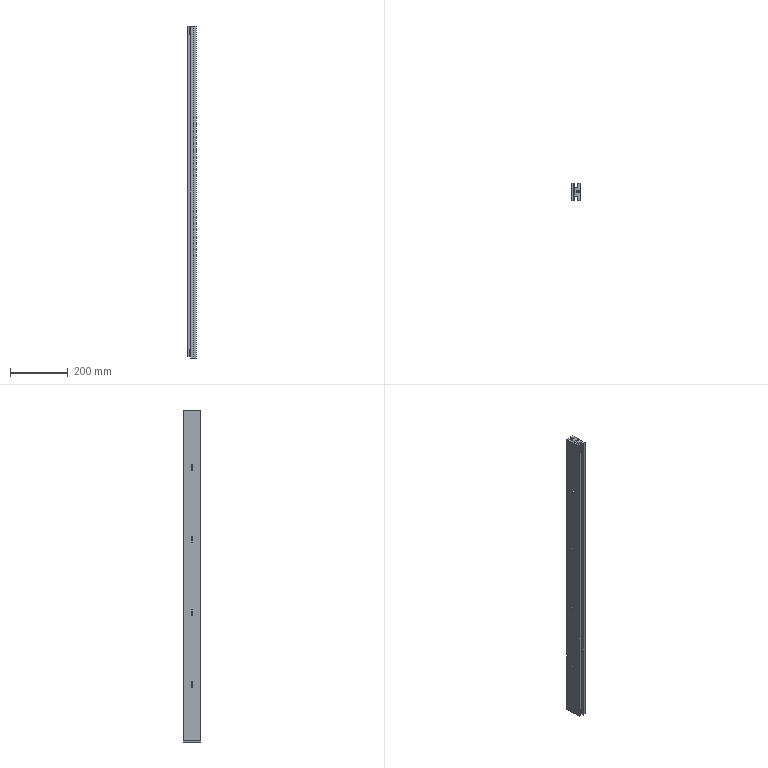Part | STEP file | 750038301 | 1 solid | 50 faces | box 30 x 60 x 1149 mm | volume 1566849 mm3 | plane 38 | cylinder 12 | commonest cylinder face diameters 6 x12
STEP:
#1=CARTESIAN_POINT('',(10.,30.,960.));
#2=VERTEX_POINT('',#1);
#3=CARTESIAN_POINT('',(10.,33.,957.));
#4=VERTEX_POINT('',#3);
#5=CARTESIAN_POINT('',(10.,30.,957.));
#6=DIRECTION('',(-1.,0.,0.));
#7=DIRECTION('',(0.,0.,1.));
#8=AXIS2_PLACEMENT_3D('',#5,#6,#7);
#9=CIRCLE('',#8,3.);
#10=EDGE_CURVE('',#2,#4,#9,.T.);
#11=ORIENTED_EDGE('',*,*,#10,.F.);
#12=CARTESIAN_POINT('',(0.,30.,960.));
#13=VERTEX_POINT('',#12);
#14=CARTESIAN_POINT('',(10.,30.,960.));
#15=DIRECTION('',(-1.,0.,0.));
#16=VECTOR('',#15,1000.);
#17=LINE('',#14,#16);
#18=EDGE_CURVE('',#2,#13,#17,.T.);
#19=ORIENTED_EDGE('',*,*,#18,.T.);
#20=CARTESIAN_POINT('',(0.,33.,957.));
#21=VERTEX_POINT('',#20);
#22=CARTESIAN_POINT('',(0.,30.,957.));
#23=DIRECTION('',(-1.,0.,0.));
#24=DIRECTION('',(0.,0.,1.));
#25=AXIS2_PLACEMENT_3D('',#22,#23,#24);
#26=CIRCLE('',#25,3.);
#27=EDGE_CURVE('',#13,#21,#26,.T.);
#28=ORIENTED_EDGE('',*,*,#27,.T.);
#29=CARTESIAN_POINT('',(10.,33.,957.));
#30=DIRECTION('',(-1.,0.,0.));
#31=VECTOR('',#30,1000.);
#32=LINE('',#29,#31);
#33=EDGE_CURVE('',#4,#21,#32,.T.);
#34=ORIENTED_EDGE('',*,*,#33,.F.);
#35=EDGE_LOOP('',(#11,#19,#28,#34));
#36=FACE_OUTER_BOUND('',#35,.T.);
#37=CARTESIAN_POINT('',(10.,30.,957.));
#38=DIRECTION('',(-1.,0.,0.));
#39=DIRECTION('',(0.,0.,1.));
#40=AXIS2_PLACEMENT_3D('',#37,#38,#39);
#41=CYLINDRICAL_SURFACE('',#40,3.);
#42=ADVANCED_FACE('',(#36),#41,.F.);
#43=CARTESIAN_POINT('',(10.,30.,710.));
#44=VERTEX_POINT('',#43);
#45=CARTESIAN_POINT('',(10.,33.,707.));
#46=VERTEX_POINT('',#45);
#47=CARTESIAN_POINT('',(10.,30.,707.));
#48=DIRECTION('',(-1.,0.,0.));
#49=DIRECTION('',(0.,0.,1.));
#50=AXIS2_PLACEMENT_3D('',#47,#48,#49);
#51=CIRCLE('',#50,3.);
#52=EDGE_CURVE('',#44,#46,#51,.T.);
#53=ORIENTED_EDGE('',*,*,#52,.F.);
#54=CARTESIAN_POINT('',(0.,30.,710.));
#55=VERTEX_POINT('',#54);
#56=CARTESIAN_POINT('',(10.,30.,710.));
#57=DIRECTION('',(-1.,0.,0.));
#58=VECTOR('',#57,1000.);
#59=LINE('',#56,#58);
#60=EDGE_CURVE('',#44,#55,#59,.T.);
#61=ORIENTED_EDGE('',*,*,#60,.T.);
#62=CARTESIAN_POINT('',(0.,33.,707.));
#63=VERTEX_POINT('',#62);
#64=CARTESIAN_POINT('',(0.,30.,707.));
#65=DIRECTION('',(-1.,0.,0.));
#66=DIRECTION('',(0.,0.,1.));
#67=AXIS2_PLACEMENT_3D('',#64,#65,#66);
#68=CIRCLE('',#67,3.);
#69=EDGE_CURVE('',#55,#63,#68,.T.);
#70=ORIENTED_EDGE('',*,*,#69,.T.);
#71=CARTESIAN_POINT('',(10.,33.,707.));
#72=DIRECTION('',(-1.,0.,0.));
#73=VECTOR('',#72,1000.);
#74=LINE('',#71,#73);
#75=EDGE_CURVE('',#46,#63,#74,.T.);
#76=ORIENTED_EDGE('',*,*,#75,.F.);
#77=EDGE_LOOP('',(#53,#61,#70,#76));
#78=FACE_OUTER_BOUND('',#77,.T.);
#79=CARTESIAN_POINT('',(10.,30.,707.));
#80=DIRECTION('',(-1.,0.,0.));
#81=DIRECTION('',(0.,0.,1.));
#82=AXIS2_PLACEMENT_3D('',#79,#80,#81);
#83=CYLINDRICAL_SURFACE('',#82,3.);
#84=ADVANCED_FACE('',(#78),#83,.F.);
#85=CARTESIAN_POINT('',(10.,30.,460.));
#86=VERTEX_POINT('',#85);
#87=CARTESIAN_POINT('',(10.,33.,457.));
#88=VERTEX_POINT('',#87);
#89=CARTESIAN_POINT('',(10.,30.,457.));
#90=DIRECTION('',(-1.,0.,0.));
#91=DIRECTION('',(0.,0.,1.));
#92=AXIS2_PLACEMENT_3D('',#89,#90,#91);
#93=CIRCLE('',#92,3.);
#94=EDGE_CURVE('',#86,#88,#93,.T.);
#95=ORIENTED_EDGE('',*,*,#94,.F.);
#96=CARTESIAN_POINT('',(0.,30.,460.));
#97=VERTEX_POINT('',#96);
#98=CARTESIAN_POINT('',(10.,30.,460.));
#99=DIRECTION('',(-1.,0.,0.));
#100=VECTOR('',#99,1000.);
#101=LINE('',#98,#100);
#102=EDGE_CURVE('',#86,#97,#101,.T.);
#103=ORIENTED_EDGE('',*,*,#102,.T.);
#104=CARTESIAN_POINT('',(0.,33.,457.));
#105=VERTEX_POINT('',#104);
#106=CARTESIAN_POINT('',(0.,30.,457.));
#107=DIRECTION('',(-1.,0.,0.));
#108=DIRECTION('',(0.,0.,1.));
#109=AXIS2_PLACEMENT_3D('',#106,#107,#108);
#110=CIRCLE('',#109,3.);
#111=EDGE_CURVE('',#97,#105,#110,.T.);
#112=ORIENTED_EDGE('',*,*,#111,.T.);
#113=CARTESIAN_POINT('',(10.,33.,457.));
#114=DIRECTION('',(-1.,0.,0.));
#115=VECTOR('',#114,1000.);
#116=LINE('',#113,#115);
#117=EDGE_CURVE('',#88,#105,#116,.T.);
#118=ORIENTED_EDGE('',*,*,#117,.F.);
#119=EDGE_LOOP('',(#95,#103,#112,#118));
#120=FACE_OUTER_BOUND('',#119,.T.);
#121=CARTESIAN_POINT('',(10.,30.,457.));
#122=DIRECTION('',(-1.,0.,0.));
#123=DIRECTION('',(0.,0.,1.));
#124=AXIS2_PLACEMENT_3D('',#121,#122,#123);
#125=CYLINDRICAL_SURFACE('',#124,3.);
#126=ADVANCED_FACE('',(#120),#125,.F.);
#127=CARTESIAN_POINT('',(10.,30.,210.));
#128=VERTEX_POINT('',#127);
#129=CARTESIAN_POINT('',(10.,33.,207.));
#130=VERTEX_POINT('',#129);
#131=CARTESIAN_POINT('',(10.,30.,207.));
#132=DIRECTION('',(-1.,0.,0.));
#133=DIRECTION('',(0.,0.,1.));
#134=AXIS2_PLACEMENT_3D('',#131,#132,#133);
#135=CIRCLE('',#134,3.);
#136=EDGE_CURVE('',#128,#130,#135,.T.);
#137=ORIENTED_EDGE('',*,*,#136,.F.);
#138=CARTESIAN_POINT('',(0.,30.,210.));
#139=VERTEX_POINT('',#138);
#140=CARTESIAN_POINT('',(10.,30.,210.));
#141=DIRECTION('',(-1.,0.,0.));
#142=VECTOR('',#141,1000.);
#143=LINE('',#140,#142);
#144=EDGE_CURVE('',#128,#139,#143,.T.);
#145=ORIENTED_EDGE('',*,*,#144,.T.);
#146=CARTESIAN_POINT('',(0.,33.,207.));
#147=VERTEX_POINT('',#146);
#148=CARTESIAN_POINT('',(0.,30.,207.));
#149=DIRECTION('',(-1.,0.,0.));
#150=DIRECTION('',(0.,0.,1.));
#151=AXIS2_PLACEMENT_3D('',#148,#149,#150);
#152=CIRCLE('',#151,3.);
#153=EDGE_CURVE('',#139,#147,#152,.T.);
#154=ORIENTED_EDGE('',*,*,#153,.T.);
#155=CARTESIAN_POINT('',(10.,33.,207.));
#156=DIRECTION('',(-1.,0.,0.));
#157=VECTOR('',#156,1000.);
#158=LINE('',#155,#157);
#159=EDGE_CURVE('',#130,#147,#158,.T.);
#160=ORIENTED_EDGE('',*,*,#159,.F.);
#161=EDGE_LOOP('',(#137,#145,#154,#160));
#162=FACE_OUTER_BOUND('',#161,.T.);
#163=CARTESIAN_POINT('',(10.,30.,207.));
#164=DIRECTION('',(-1.,0.,0.));
#165=DIRECTION('',(0.,0.,1.));
#166=AXIS2_PLACEMENT_3D('',#163,#164,#165);
#167=CYLINDRICAL_SURFACE('',#166,3.);
#168=ADVANCED_FACE('',(#162),#167,.F.);
#169=CARTESIAN_POINT('',(0.,0.,1149.));
#170=VERTEX_POINT('',#169);
#171=CARTESIAN_POINT('',(0.,0.,5.));
#172=VERTEX_POINT('',#171);
#173=CARTESIAN_POINT('',(0.,0.,1149.));
#174=DIRECTION('',(0.,0.,-1.));
#175=VECTOR('',#174,1000.);
#176=LINE('',#173,#175);
#177=EDGE_CURVE('',#170,#172,#176,.T.);
#178=ORIENTED_EDGE('',*,*,#177,.F.);
#179=CARTESIAN_POINT('',(0.,60.,1149.));
#180=VERTEX_POINT('',#179);
#181=CARTESIAN_POINT('',(0.,60.,1149.));
#182=DIRECTION('',(0.,-1.,0.));
#183=VECTOR('',#182,1000.);
#184=LINE('',#181,#183);
#185=EDGE_CURVE('',#180,#170,#184,.T.);
#186=ORIENTED_EDGE('',*,*,#185,.F.);
#187=CARTESIAN_POINT('',(0.,60.,5.));
#188=VERTEX_POINT('',#187);
#189=CARTESIAN_POINT('',(0.,60.,1149.));
#190=DIRECTION('',(0.,0.,1.));
#191=VECTOR('',#190,1000.);
#192=LINE('',#189,#191);
#193=EDGE_CURVE('',#188,#180,#192,.T.);
#194=ORIENTED_EDGE('',*,*,#193,.F.);
#195=CARTESIAN_POINT('',(0.,60.,5.));
#196=DIRECTION('',(0.,1.,0.));
#197=VECTOR('',#196,1000.);
#198=LINE('',#195,#197);
#199=EDGE_CURVE('',#172,#188,#198,.T.);
#200=ORIENTED_EDGE('',*,*,#199,.F.);
#201=EDGE_LOOP('',(#178,#186,#194,#200));
#202=FACE_OUTER_BOUND('',#201,.T.);
#203=CARTESIAN_POINT('',(0.,27.,942.));
#204=VERTEX_POINT('',#203);
#205=CARTESIAN_POINT('',(0.,27.,957.));
#206=VERTEX_POINT('',#205);
#207=CARTESIAN_POINT('',(0.,27.,1149.));
#208=DIRECTION('',(0.,0.,1.));
#209=VECTOR('',#208,1000.);
#210=LINE('',#207,#209);
#211=EDGE_CURVE('',#204,#206,#210,.T.);
#212=ORIENTED_EDGE('',*,*,#211,.F.);
#213=CARTESIAN_POINT('',(0.,33.,942.));
#214=VERTEX_POINT('',#213);
#215=CARTESIAN_POINT('',(0.,30.,942.));
#216=DIRECTION('',(-1.,0.,0.));
#217=DIRECTION('',(0.,0.,1.));
#218=AXIS2_PLACEMENT_3D('',#215,#216,#217);
#219=CIRCLE('',#218,3.);
#220=EDGE_CURVE('',#214,#204,#219,.T.);
#221=ORIENTED_EDGE('',*,*,#220,.F.);
#222=CARTESIAN_POINT('',(0.,33.,1149.));
#223=DIRECTION('',(0.,0.,-1.));
#224=VECTOR('',#223,1000.);
#225=LINE('',#222,#224);
#226=EDGE_CURVE('',#21,#214,#225,.T.);
#227=ORIENTED_EDGE('',*,*,#226,.F.);
#228=ORIENTED_EDGE('',*,*,#27,.F.);
#229=CARTESIAN_POINT('',(0.,30.,957.));
#230=DIRECTION('',(-1.,0.,0.));
#231=DIRECTION('',(0.,0.,1.));
#232=AXIS2_PLACEMENT_3D('',#229,#230,#231);
#233=CIRCLE('',#232,3.);
#234=EDGE_CURVE('',#206,#13,#233,.T.);
#235=ORIENTED_EDGE('',*,*,#234,.F.);
#236=EDGE_LOOP('',(#212,#221,#227,#228,#235));
#237=FACE_BOUND('',#236,.T.);
#238=CARTESIAN_POINT('',(0.,27.,692.));
#239=VERTEX_POINT('',#238);
#240=CARTESIAN_POINT('',(0.,27.,707.));
#241=VERTEX_POINT('',#240);
#242=CARTESIAN_POINT('',(0.,27.,1149.));
#243=DIRECTION('',(0.,0.,1.));
#244=VECTOR('',#243,1000.);
#245=LINE('',#242,#244);
#246=EDGE_CURVE('',#239,#241,#245,.T.);
#247=ORIENTED_EDGE('',*,*,#246,.F.);
#248=CARTESIAN_POINT('',(0.,33.,692.));
#249=VERTEX_POINT('',#248);
#250=CARTESIAN_POINT('',(0.,30.,692.));
#251=DIRECTION('',(-1.,0.,0.));
#252=DIRECTION('',(0.,0.,1.));
#253=AXIS2_PLACEMENT_3D('',#250,#251,#252);
#254=CIRCLE('',#253,3.);
#255=EDGE_CURVE('',#249,#239,#254,.T.);
#256=ORIENTED_EDGE('',*,*,#255,.F.);
#257=CARTESIAN_POINT('',(0.,33.,1149.));
#258=DIRECTION('',(0.,0.,-1.));
#259=VECTOR('',#258,1000.);
#260=LINE('',#257,#259);
#261=EDGE_CURVE('',#63,#249,#260,.T.);
#262=ORIENTED_EDGE('',*,*,#261,.F.);
#263=ORIENTED_EDGE('',*,*,#69,.F.);
#264=CARTESIAN_POINT('',(0.,30.,707.));
#265=DIRECTION('',(-1.,0.,0.));
#266=DIRECTION('',(0.,0.,1.));
#267=AXIS2_PLACEMENT_3D('',#264,#265,#266);
#268=CIRCLE('',#267,3.);
#269=EDGE_CURVE('',#241,#55,#268,.T.);
#270=ORIENTED_EDGE('',*,*,#269,.F.);
#271=EDGE_LOOP('',(#247,#256,#262,#263,#270));
#272=FACE_BOUND('',#271,.T.);
#273=CARTESIAN_POINT('',(0.,27.,442.));
#274=VERTEX_POINT('',#273);
#275=CARTESIAN_POINT('',(0.,27.,457.));
#276=VERTEX_POINT('',#275);
#277=CARTESIAN_POINT('',(0.,27.,1149.));
#278=DIRECTION('',(0.,0.,1.));
#279=VECTOR('',#278,1000.);
#280=LINE('',#277,#279);
#281=EDGE_CURVE('',#274,#276,#280,.T.);
#282=ORIENTED_EDGE('',*,*,#281,.F.);
#283=CARTESIAN_POINT('',(0.,33.,442.));
#284=VERTEX_POINT('',#283);
#285=CARTESIAN_POINT('',(0.,30.,442.));
#286=DIRECTION('',(-1.,0.,0.));
#287=DIRECTION('',(0.,0.,1.));
#288=AXIS2_PLACEMENT_3D('',#285,#286,#287);
#289=CIRCLE('',#288,3.);
#290=EDGE_CURVE('',#284,#274,#289,.T.);
#291=ORIENTED_EDGE('',*,*,#290,.F.);
#292=CARTESIAN_POINT('',(0.,33.,1149.));
#293=DIRECTION('',(0.,0.,-1.));
#294=VECTOR('',#293,1000.);
#295=LINE('',#292,#294);
#296=EDGE_CURVE('',#105,#284,#295,.T.);
#297=ORIENTED_EDGE('',*,*,#296,.F.);
#298=ORIENTED_EDGE('',*,*,#111,.F.);
#299=CARTESIAN_POINT('',(0.,30.,457.));
#300=DIRECTION('',(-1.,0.,0.));
#301=DIRECTION('',(0.,0.,1.));
#302=AXIS2_PLACEMENT_3D('',#299,#300,#301);
#303=CIRCLE('',#302,3.);
#304=EDGE_CURVE('',#276,#97,#303,.T.);
#305=ORIENTED_EDGE('',*,*,#304,.F.);
#306=EDGE_LOOP('',(#282,#291,#297,#298,#305));
#307=FACE_BOUND('',#306,.T.);
#308=CARTESIAN_POINT('',(0.,27.,192.));
#309=VERTEX_POINT('',#308);
#310=CARTESIAN_POINT('',(0.,27.,207.));
#311=VERTEX_POINT('',#310);
#312=CARTESIAN_POINT('',(0.,27.,1149.));
#313=DIRECTION('',(0.,0.,1.));
#314=VECTOR('',#313,1000.);
#315=LINE('',#312,#314);
#316=EDGE_CURVE('',#309,#311,#315,.T.);
#317=ORIENTED_EDGE('',*,*,#316,.F.);
#318=CARTESIAN_POINT('',(0.,33.,192.));
#319=VERTEX_POINT('',#318);
#320=CARTESIAN_POINT('',(0.,30.,192.));
#321=DIRECTION('',(-1.,0.,0.));
#322=DIRECTION('',(0.,0.,1.));
#323=AXIS2_PLACEMENT_3D('',#320,#321,#322);
#324=CIRCLE('',#323,3.);
#325=EDGE_CURVE('',#319,#309,#324,.T.);
#326=ORIENTED_EDGE('',*,*,#325,.F.);
#327=CARTESIAN_POINT('',(0.,33.,1149.));
#328=DIRECTION('',(0.,0.,-1.));
#329=VECTOR('',#328,1000.);
#330=LINE('',#327,#329);
#331=EDGE_CURVE('',#147,#319,#330,.T.);
#332=ORIENTED_EDGE('',*,*,#331,.F.);
#333=ORIENTED_EDGE('',*,*,#153,.F.);
#334=CARTESIAN_POINT('',(0.,30.,207.));
#335=DIRECTION('',(-1.,0.,0.));
#336=DIRECTION('',(0.,0.,1.));
#337=AXIS2_PLACEMENT_3D('',#334,#335,#336);
#338=CIRCLE('',#337,3.);
#339=EDGE_CURVE('',#311,#139,#338,.T.);
#340=ORIENTED_EDGE('',*,*,#339,.F.);
#341=EDGE_LOOP('',(#317,#326,#332,#333,#340));
#342=FACE_BOUND('',#341,.T.);
#343=CARTESIAN_POINT('',(0.,60.,1149.));
#344=DIRECTION('',(1.,0.,0.));
#345=DIRECTION('',(0.,0.,-1.));
#346=AXIS2_PLACEMENT_3D('',#343,#344,#345);
#347=PLANE('',#346);
#348=ADVANCED_FACE('',(#202,#237,#272,#307,#342),#347,.F.);
#349=CARTESIAN_POINT('',(6.5,0.,5.));
#350=VERTEX_POINT('',#349);
#351=CARTESIAN_POINT('',(10.,0.,5.));
#352=DIRECTION('',(1.,0.,0.));
#353=VECTOR('',#352,1000.);
#354=LINE('',#351,#353);
#355=EDGE_CURVE('',#172,#350,#354,.T.);
#356=ORIENTED_EDGE('',*,*,#355,.F.);
#357=ORIENTED_EDGE('',*,*,#199,.T.);
#358=CARTESIAN_POINT('',(6.5,60.,5.));
#359=VERTEX_POINT('',#358);
#360=CARTESIAN_POINT('',(10.,60.,5.));
#361=DIRECTION('',(-1.,0.,0.));
#362=VECTOR('',#361,1000.);
#363=LINE('',#360,#362);
#364=EDGE_CURVE('',#359,#188,#363,.T.);
#365=ORIENTED_EDGE('',*,*,#364,.F.);
#366=CARTESIAN_POINT('',(6.5,0.,5.));
#367=DIRECTION('',(0.,1.,0.));
#368=VECTOR('',#367,1000.);
#369=LINE('',#366,#368);
#370=EDGE_CURVE('',#350,#359,#369,.T.);
#371=ORIENTED_EDGE('',*,*,#370,.F.);
#372=EDGE_LOOP('',(#356,#357,#365,#371));
#373=FACE_OUTER_BOUND('',#372,.T.);
#374=CARTESIAN_POINT('',(10.,0.,5.));
#375=DIRECTION('',(0.,0.,1.));
#376=DIRECTION('',(0.,-1.,0.));
#377=AXIS2_PLACEMENT_3D('',#374,#375,#376);
#378=PLANE('',#377);
#379=ADVANCED_FACE('',(#373),#378,.F.);
#380=CARTESIAN_POINT('',(6.5,0.,1118.));
#381=VERTEX_POINT('',#380);
#382=CARTESIAN_POINT('',(9.5,0.,1118.));
#383=VERTEX_POINT('',#382);
#384=CARTESIAN_POINT('',(0.,0.,1118.));
#385=DIRECTION('',(1.,0.,0.));
#386=VECTOR('',#385,1000.);
#387=LINE('',#384,#386);
#388=EDGE_CURVE('',#381,#383,#387,.T.);
#389=ORIENTED_EDGE('',*,*,#388,.F.);
#390=CARTESIAN_POINT('',(6.5,0.,1149.));
#391=VERTEX_POINT('',#390);
#392=CARTESIAN_POINT('',(6.5,0.,1149.));
#393=DIRECTION('',(0.,0.,-1.));
#394=VECTOR('',#393,1000.);
#395=LINE('',#392,#394);
#396=EDGE_CURVE('',#391,#381,#395,.T.);
#397=ORIENTED_EDGE('',*,*,#396,.F.);
#398=CARTESIAN_POINT('',(0.,0.,1149.));
#399=DIRECTION('',(1.,0.,0.));
#400=VECTOR('',#399,1000.);
#401=LINE('',#398,#400);
#402=EDGE_CURVE('',#170,#391,#401,.T.);
#403=ORIENTED_EDGE('',*,*,#402,.F.);
#404=ORIENTED_EDGE('',*,*,#177,.T.);
#405=ORIENTED_EDGE('',*,*,#355,.T.);
#406=CARTESIAN_POINT('',(6.5,0.,31.));
#407=VERTEX_POINT('',#406);
#408=CARTESIAN_POINT('',(6.5,0.,1149.));
#409=DIRECTION('',(0.,0.,-1.));
#410=VECTOR('',#409,1000.);
#411=LINE('',#408,#410);
#412=EDGE_CURVE('',#407,#350,#411,.T.);
#413=ORIENTED_EDGE('',*,*,#412,.F.);
#414=CARTESIAN_POINT('',(9.5,0.,31.));
#415=VERTEX_POINT('',#414);
#416=CARTESIAN_POINT('',(0.,0.,31.));
#417=DIRECTION('',(-1.,0.,0.));
#418=VECTOR('',#417,1000.);
#419=LINE('',#416,#418);
#420=EDGE_CURVE('',#415,#407,#419,.T.);
#421=ORIENTED_EDGE('',*,*,#420,.F.);
#422=CARTESIAN_POINT('',(9.5,0.,1149.));
#423=DIRECTION('',(0.,0.,-1.));
#424=VECTOR('',#423,1000.);
#425=LINE('',#422,#424);
#426=EDGE_CURVE('',#383,#415,#425,.T.);
#427=ORIENTED_EDGE('',*,*,#426,.F.);
#428=EDGE_LOOP('',(#389,#397,#403,#404,#405,#413,#421,#427));
#429=FACE_OUTER_BOUND('',#428,.T.);
#430=CARTESIAN_POINT('',(0.,0.,1149.));
#431=DIRECTION('',(0.,1.,0.));
#432=DIRECTION('',(0.,0.,1.));
#433=AXIS2_PLACEMENT_3D('',#430,#431,#432);
#434=PLANE('',#433);
#435=ADVANCED_FACE('',(#429),#434,.F.);
#436=CARTESIAN_POINT('',(6.5,60.,1149.));
#437=VERTEX_POINT('',#436);
#438=CARTESIAN_POINT('',(0.,60.,1149.));
#439=DIRECTION('',(-1.,0.,0.));
#440=VECTOR('',#439,1000.);
#441=LINE('',#438,#440);
#442=EDGE_CURVE('',#437,#180,#441,.T.);
#443=ORIENTED_EDGE('',*,*,#442,.T.);
#444=ORIENTED_EDGE('',*,*,#185,.T.);
#445=ORIENTED_EDGE('',*,*,#402,.T.);
#446=CARTESIAN_POINT('',(6.5,0.,1149.));
#447=DIRECTION('',(0.,1.,0.));
#448=VECTOR('',#447,1000.);
#449=LINE('',#446,#448);
#450=EDGE_CURVE('',#391,#437,#449,.T.);
#451=ORIENTED_EDGE('',*,*,#450,.T.);
#452=EDGE_LOOP('',(#443,#444,#445,#451));
#453=FACE_OUTER_BOUND('',#452,.T.);
#454=CARTESIAN_POINT('',(0.,0.,1149.));
#455=DIRECTION('',(0.,0.,1.));
#456=DIRECTION('',(1.,0.,0.));
#457=AXIS2_PLACEMENT_3D('',#454,#455,#456);
#458=PLANE('',#457);
#459=ADVANCED_FACE('',(#453),#458,.T.);
#460=CARTESIAN_POINT('',(9.5,60.,1118.));
#461=VERTEX_POINT('',#460);
#462=CARTESIAN_POINT('',(6.5,60.,1118.));
#463=VERTEX_POINT('',#462);
#464=CARTESIAN_POINT('',(9.5,60.,1118.));
#465=DIRECTION('',(-1.,0.,0.));
#466=VECTOR('',#465,1000.);
#467=LINE('',#464,#466);
#468=EDGE_CURVE('',#461,#463,#467,.T.);
#469=ORIENTED_EDGE('',*,*,#468,.F.);
#470=CARTESIAN_POINT('',(9.5,60.,31.));
#471=VERTEX_POINT('',#470);
#472=CARTESIAN_POINT('',(9.5,60.,1149.));
#473=DIRECTION('',(0.,0.,1.));
#474=VECTOR('',#473,1000.);
#475=LINE('',#472,#474);
#476=EDGE_CURVE('',#471,#461,#475,.T.);
#477=ORIENTED_EDGE('',*,*,#476,.F.);
#478=CARTESIAN_POINT('',(6.5,60.,31.));
#479=VERTEX_POINT('',#478);
#480=CARTESIAN_POINT('',(9.5,60.,31.));
#481=DIRECTION('',(1.,0.,0.));
#482=VECTOR('',#481,1000.);
#483=LINE('',#480,#482);
#484=EDGE_CURVE('',#479,#471,#483,.T.);
#485=ORIENTED_EDGE('',*,*,#484,.F.);
#486=CARTESIAN_POINT('',(6.5,60.,1149.));
#487=DIRECTION('',(0.,0.,1.));
#488=VECTOR('',#487,1000.);
#489=LINE('',#486,#488);
#490=EDGE_CURVE('',#359,#479,#489,.T.);
#491=ORIENTED_EDGE('',*,*,#490,.F.);
#492=ORIENTED_EDGE('',*,*,#364,.T.);
#493=ORIENTED_EDGE('',*,*,#193,.T.);
#494=ORIENTED_EDGE('',*,*,#442,.F.);
#495=CARTESIAN_POINT('',(6.5,60.,1149.));
#496=DIRECTION('',(0.,0.,1.));
#497=VECTOR('',#496,1000.);
#498=LINE('',#495,#497);
#499=EDGE_CURVE('',#463,#437,#498,.T.);
#500=ORIENTED_EDGE('',*,*,#499,.F.);
#501=EDGE_LOOP('',(#469,#477,#485,#491,#492,#493,#494,#500));
#502=FACE_OUTER_BOUND('',#501,.T.);
#503=CARTESIAN_POINT('',(9.5,60.,1149.));
#504=DIRECTION('',(0.,-1.,0.));
#505=DIRECTION('',(0.,0.,-1.));
#506=AXIS2_PLACEMENT_3D('',#503,#504,#505);
#507=PLANE('',#506);
#508=ADVANCED_FACE('',(#502),#507,.F.);
#509=ORIENTED_EDGE('',*,*,#18,.F.);
#510=CARTESIAN_POINT('',(10.,27.,957.));
#511=VERTEX_POINT('',#510);
#512=CARTESIAN_POINT('',(10.,30.,957.));
#513=DIRECTION('',(-1.,0.,0.));
#514=DIRECTION('',(0.,0.,1.));
#515=AXIS2_PLACEMENT_3D('',#512,#513,#514);
#516=CIRCLE('',#515,3.);
#517=EDGE_CURVE('',#511,#2,#516,.T.);
#518=ORIENTED_EDGE('',*,*,#517,.F.);
#519=CARTESIAN_POINT('',(10.,27.,957.));
#520=DIRECTION('',(1.,0.,0.));
#521=VECTOR('',#520,1000.);
#522=LINE('',#519,#521);
#523=EDGE_CURVE('',#206,#511,#522,.T.);
#524=ORIENTED_EDGE('',*,*,#523,.F.);
#525=ORIENTED_EDGE('',*,*,#234,.T.);
#526=EDGE_LOOP('',(#509,#518,#524,#525));
#527=FACE_OUTER_BOUND('',#526,.T.);
#528=CARTESIAN_POINT('',(10.,30.,957.));
#529=DIRECTION('',(-1.,0.,0.));
#530=DIRECTION('',(0.,0.,1.));
#531=AXIS2_PLACEMENT_3D('',#528,#529,#530);
#532=CYLINDRICAL_SURFACE('',#531,3.);
#533=ADVANCED_FACE('',(#527),#532,.F.);
#534=ORIENTED_EDGE('',*,*,#523,.T.);
#535=CARTESIAN_POINT('',(10.,27.,942.));
#536=VERTEX_POINT('',#535);
#537=CARTESIAN_POINT('',(10.,27.,942.));
#538=DIRECTION('',(0.,0.,1.));
#539=VECTOR('',#538,1000.);
#540=LINE('',#537,#539);
#541=EDGE_CURVE('',#536,#511,#540,.T.);
#542=ORIENTED_EDGE('',*,*,#541,.F.);
#543=CARTESIAN_POINT('',(10.,27.,942.));
#544=DIRECTION('',(1.,0.,0.));
#545=VECTOR('',#544,1000.);
#546=LINE('',#543,#545);
#547=EDGE_CURVE('',#204,#536,#546,.T.);
#548=ORIENTED_EDGE('',*,*,#547,.F.);
#549=ORIENTED_EDGE('',*,*,#211,.T.);
#550=EDGE_LOOP('',(#534,#542,#548,#549));
#551=FACE_OUTER_BOUND('',#550,.T.);
#552=CARTESIAN_POINT('',(10.,27.,942.));
#553=DIRECTION('',(0.,-1.,0.));
#554=DIRECTION('',(0.,0.,-1.));
#555=AXIS2_PLACEMENT_3D('',#552,#553,#554);
#556=PLANE('',#555);
#557=ADVANCED_FACE('',(#551),#556,.F.);
#558=ORIENTED_EDGE('',*,*,#547,.T.);
#559=CARTESIAN_POINT('',(10.,33.,942.));
#560=VERTEX_POINT('',#559);
#561=CARTESIAN_POINT('',(10.,30.,942.));
#562=DIRECTION('',(-1.,0.,0.));
#563=DIRECTION('',(0.,0.,1.));
#564=AXIS2_PLACEMENT_3D('',#561,#562,#563);
#565=CIRCLE('',#564,3.);
#566=EDGE_CURVE('',#560,#536,#565,.T.);
#567=ORIENTED_EDGE('',*,*,#566,.F.);
#568=CARTESIAN_POINT('',(10.,33.,942.));
#569=DIRECTION('',(1.,0.,0.));
#570=VECTOR('',#569,1000.);
#571=LINE('',#568,#570);
#572=EDGE_CURVE('',#214,#560,#571,.T.);
#573=ORIENTED_EDGE('',*,*,#572,.F.);
#574=ORIENTED_EDGE('',*,*,#220,.T.);
#575=EDGE_LOOP('',(#558,#567,#573,#574));
#576=FACE_OUTER_BOUND('',#575,.T.);
#577=CARTESIAN_POINT('',(10.,30.,942.));
#578=DIRECTION('',(-1.,0.,0.));
#579=DIRECTION('',(0.,0.,1.));
#580=AXIS2_PLACEMENT_3D('',#577,#578,#579);
#581=CYLINDRICAL_SURFACE('',#580,3.);
#582=ADVANCED_FACE('',(#576),#581,.F.);
#583=ORIENTED_EDGE('',*,*,#572,.T.);
#584=CARTESIAN_POINT('',(10.,33.,957.));
#585=DIRECTION('',(0.,0.,-1.));
#586=VECTOR('',#585,1000.);
#587=LINE('',#584,#586);
#588=EDGE_CURVE('',#4,#560,#587,.T.);
#589=ORIENTED_EDGE('',*,*,#588,.F.);
#590=ORIENTED_EDGE('',*,*,#33,.T.);
#591=ORIENTED_EDGE('',*,*,#226,.T.);
#592=EDGE_LOOP('',(#583,#589,#590,#591));
#593=FACE_OUTER_BOUND('',#592,.T.);
#594=CARTESIAN_POINT('',(10.,33.,957.));
#595=DIRECTION('',(0.,1.,0.));
#596=DIRECTION('',(0.,0.,1.));
#597=AXIS2_PLACEMENT_3D('',#594,#595,#596);
#598=PLANE('',#597);
#599=ADVANCED_FACE('',(#593),#598,.F.);
#600=ORIENTED_EDGE('',*,*,#60,.F.);
#601=CARTESIAN_POINT('',(10.,27.,707.));
#602=VERTEX_POINT('',#601);
#603=CARTESIAN_POINT('',(10.,30.,707.));
#604=DIRECTION('',(-1.,0.,0.));
#605=DIRECTION('',(0.,0.,1.));
#606=AXIS2_PLACEMENT_3D('',#603,#604,#605);
#607=CIRCLE('',#606,3.);
#608=EDGE_CURVE('',#602,#44,#607,.T.);
#609=ORIENTED_EDGE('',*,*,#608,.F.);
#610=CARTESIAN_POINT('',(10.,27.,707.));
#611=DIRECTION('',(1.,0.,0.));
#612=VECTOR('',#611,1000.);
#613=LINE('',#610,#612);
#614=EDGE_CURVE('',#241,#602,#613,.T.);
#615=ORIENTED_EDGE('',*,*,#614,.F.);
#616=ORIENTED_EDGE('',*,*,#269,.T.);
#617=EDGE_LOOP('',(#600,#609,#615,#616));
#618=FACE_OUTER_BOUND('',#617,.T.);
#619=CARTESIAN_POINT('',(10.,30.,707.));
#620=DIRECTION('',(-1.,0.,0.));
#621=DIRECTION('',(0.,0.,1.));
#622=AXIS2_PLACEMENT_3D('',#619,#620,#621);
#623=CYLINDRICAL_SURFACE('',#622,3.);
#624=ADVANCED_FACE('',(#618),#623,.F.);
#625=ORIENTED_EDGE('',*,*,#614,.T.);
#626=CARTESIAN_POINT('',(10.,27.,692.));
#627=VERTEX_POINT('',#626);
#628=CARTESIAN_POINT('',(10.,27.,692.));
#629=DIRECTION('',(0.,0.,1.));
#630=VECTOR('',#629,1000.);
#631=LINE('',#628,#630);
#632=EDGE_CURVE('',#627,#602,#631,.T.);
#633=ORIENTED_EDGE('',*,*,#632,.F.);
#634=CARTESIAN_POINT('',(10.,27.,692.));
#635=DIRECTION('',(1.,0.,0.));
#636=VECTOR('',#635,1000.);
#637=LINE('',#634,#636);
#638=EDGE_CURVE('',#239,#627,#637,.T.);
#639=ORIENTED_EDGE('',*,*,#638,.F.);
#640=ORIENTED_EDGE('',*,*,#246,.T.);
#641=EDGE_LOOP('',(#625,#633,#639,#640));
#642=FACE_OUTER_BOUND('',#641,.T.);
#643=CARTESIAN_POINT('',(10.,27.,692.));
#644=DIRECTION('',(0.,-1.,0.));
#645=DIRECTION('',(0.,0.,-1.));
#646=AXIS2_PLACEMENT_3D('',#643,#644,#645);
#647=PLANE('',#646);
#648=ADVANCED_FACE('',(#642),#647,.F.);
#649=ORIENTED_EDGE('',*,*,#638,.T.);
#650=CARTESIAN_POINT('',(10.,33.,692.));
#651=VERTEX_POINT('',#650);
#652=CARTESIAN_POINT('',(10.,30.,692.));
#653=DIRECTION('',(-1.,0.,0.));
#654=DIRECTION('',(0.,0.,1.));
#655=AXIS2_PLACEMENT_3D('',#652,#653,#654);
#656=CIRCLE('',#655,3.);
#657=EDGE_CURVE('',#651,#627,#656,.T.);
#658=ORIENTED_EDGE('',*,*,#657,.F.);
#659=CARTESIAN_POINT('',(10.,33.,692.));
#660=DIRECTION('',(1.,0.,0.));
#661=VECTOR('',#660,1000.);
#662=LINE('',#659,#661);
#663=EDGE_CURVE('',#249,#651,#662,.T.);
#664=ORIENTED_EDGE('',*,*,#663,.F.);
#665=ORIENTED_EDGE('',*,*,#255,.T.);
#666=EDGE_LOOP('',(#649,#658,#664,#665));
#667=FACE_OUTER_BOUND('',#666,.T.);
#668=CARTESIAN_POINT('',(10.,30.,692.));
#669=DIRECTION('',(-1.,0.,0.));
#670=DIRECTION('',(0.,0.,1.));
#671=AXIS2_PLACEMENT_3D('',#668,#669,#670);
#672=CYLINDRICAL_SURFACE('',#671,3.);
#673=ADVANCED_FACE('',(#667),#672,.F.);
#674=ORIENTED_EDGE('',*,*,#663,.T.);
#675=CARTESIAN_POINT('',(10.,33.,707.));
#676=DIRECTION('',(0.,0.,-1.));
#677=VECTOR('',#676,1000.);
#678=LINE('',#675,#677);
#679=EDGE_CURVE('',#46,#651,#678,.T.);
#680=ORIENTED_EDGE('',*,*,#679,.F.);
#681=ORIENTED_EDGE('',*,*,#75,.T.);
#682=ORIENTED_EDGE('',*,*,#261,.T.);
#683=EDGE_LOOP('',(#674,#680,#681,#682));
#684=FACE_OUTER_BOUND('',#683,.T.);
#685=CARTESIAN_POINT('',(10.,33.,707.));
#686=DIRECTION('',(0.,1.,0.));
#687=DIRECTION('',(0.,0.,1.));
#688=AXIS2_PLACEMENT_3D('',#685,#686,#687);
#689=PLANE('',#688);
#690=ADVANCED_FACE('',(#684),#689,.F.);
#691=ORIENTED_EDGE('',*,*,#102,.F.);
#692=CARTESIAN_POINT('',(10.,27.,457.));
#693=VERTEX_POINT('',#692);
#694=CARTESIAN_POINT('',(10.,30.,457.));
#695=DIRECTION('',(-1.,0.,0.));
#696=DIRECTION('',(0.,0.,1.));
#697=AXIS2_PLACEMENT_3D('',#694,#695,#696);
#698=CIRCLE('',#697,3.);
#699=EDGE_CURVE('',#693,#86,#698,.T.);
#700=ORIENTED_EDGE('',*,*,#699,.F.);
#701=CARTESIAN_POINT('',(10.,27.,457.));
#702=DIRECTION('',(1.,0.,0.));
#703=VECTOR('',#702,1000.);
#704=LINE('',#701,#703);
#705=EDGE_CURVE('',#276,#693,#704,.T.);
#706=ORIENTED_EDGE('',*,*,#705,.F.);
#707=ORIENTED_EDGE('',*,*,#304,.T.);
#708=EDGE_LOOP('',(#691,#700,#706,#707));
#709=FACE_OUTER_BOUND('',#708,.T.);
#710=CARTESIAN_POINT('',(10.,30.,457.));
#711=DIRECTION('',(-1.,0.,0.));
#712=DIRECTION('',(0.,0.,1.));
#713=AXIS2_PLACEMENT_3D('',#710,#711,#712);
#714=CYLINDRICAL_SURFACE('',#713,3.);
#715=ADVANCED_FACE('',(#709),#714,.F.);
#716=ORIENTED_EDGE('',*,*,#705,.T.);
#717=CARTESIAN_POINT('',(10.,27.,442.));
#718=VERTEX_POINT('',#717);
#719=CARTESIAN_POINT('',(10.,27.,442.));
#720=DIRECTION('',(0.,0.,1.));
#721=VECTOR('',#720,1000.);
#722=LINE('',#719,#721);
#723=EDGE_CURVE('',#718,#693,#722,.T.);
#724=ORIENTED_EDGE('',*,*,#723,.F.);
#725=CARTESIAN_POINT('',(10.,27.,442.));
#726=DIRECTION('',(1.,0.,0.));
#727=VECTOR('',#726,1000.);
#728=LINE('',#725,#727);
#729=EDGE_CURVE('',#274,#718,#728,.T.);
#730=ORIENTED_EDGE('',*,*,#729,.F.);
#731=ORIENTED_EDGE('',*,*,#281,.T.);
#732=EDGE_LOOP('',(#716,#724,#730,#731));
#733=FACE_OUTER_BOUND('',#732,.T.);
#734=CARTESIAN_POINT('',(10.,27.,442.));
#735=DIRECTION('',(0.,-1.,0.));
#736=DIRECTION('',(0.,0.,-1.));
#737=AXIS2_PLACEMENT_3D('',#734,#735,#736);
#738=PLANE('',#737);
#739=ADVANCED_FACE('',(#733),#738,.F.);
#740=ORIENTED_EDGE('',*,*,#729,.T.);
#741=CARTESIAN_POINT('',(10.,33.,442.));
#742=VERTEX_POINT('',#741);
#743=CARTESIAN_POINT('',(10.,30.,442.));
#744=DIRECTION('',(-1.,0.,0.));
#745=DIRECTION('',(0.,0.,1.));
#746=AXIS2_PLACEMENT_3D('',#743,#744,#745);
#747=CIRCLE('',#746,3.);
#748=EDGE_CURVE('',#742,#718,#747,.T.);
#749=ORIENTED_EDGE('',*,*,#748,.F.);
#750=CARTESIAN_POINT('',(10.,33.,442.));
#751=DIRECTION('',(1.,0.,0.));
#752=VECTOR('',#751,1000.);
#753=LINE('',#750,#752);
#754=EDGE_CURVE('',#284,#742,#753,.T.);
#755=ORIENTED_EDGE('',*,*,#754,.F.);
#756=ORIENTED_EDGE('',*,*,#290,.T.);
#757=EDGE_LOOP('',(#740,#749,#755,#756));
#758=FACE_OUTER_BOUND('',#757,.T.);
#759=CARTESIAN_POINT('',(10.,30.,442.));
#760=DIRECTION('',(-1.,0.,0.));
#761=DIRECTION('',(0.,0.,1.));
#762=AXIS2_PLACEMENT_3D('',#759,#760,#761);
#763=CYLINDRICAL_SURFACE('',#762,3.);
#764=ADVANCED_FACE('',(#758),#763,.F.);
#765=ORIENTED_EDGE('',*,*,#754,.T.);
#766=CARTESIAN_POINT('',(10.,33.,457.));
#767=DIRECTION('',(0.,0.,-1.));
#768=VECTOR('',#767,1000.);
#769=LINE('',#766,#768);
#770=EDGE_CURVE('',#88,#742,#769,.T.);
#771=ORIENTED_EDGE('',*,*,#770,.F.);
#772=ORIENTED_EDGE('',*,*,#117,.T.);
#773=ORIENTED_EDGE('',*,*,#296,.T.);
#774=EDGE_LOOP('',(#765,#771,#772,#773));
#775=FACE_OUTER_BOUND('',#774,.T.);
#776=CARTESIAN_POINT('',(10.,33.,457.));
#777=DIRECTION('',(0.,1.,0.));
#778=DIRECTION('',(0.,0.,1.));
#779=AXIS2_PLACEMENT_3D('',#776,#777,#778);
#780=PLANE('',#779);
#781=ADVANCED_FACE('',(#775),#780,.F.);
#782=ORIENTED_EDGE('',*,*,#144,.F.);
#783=CARTESIAN_POINT('',(10.,27.,207.));
#784=VERTEX_POINT('',#783);
#785=CARTESIAN_POINT('',(10.,30.,207.));
#786=DIRECTION('',(-1.,0.,0.));
#787=DIRECTION('',(0.,0.,1.));
#788=AXIS2_PLACEMENT_3D('',#785,#786,#787);
#789=CIRCLE('',#788,3.);
#790=EDGE_CURVE('',#784,#128,#789,.T.);
#791=ORIENTED_EDGE('',*,*,#790,.F.);
#792=CARTESIAN_POINT('',(10.,27.,207.));
#793=DIRECTION('',(1.,0.,0.));
#794=VECTOR('',#793,1000.);
#795=LINE('',#792,#794);
#796=EDGE_CURVE('',#311,#784,#795,.T.);
#797=ORIENTED_EDGE('',*,*,#796,.F.);
#798=ORIENTED_EDGE('',*,*,#339,.T.);
#799=EDGE_LOOP('',(#782,#791,#797,#798));
#800=FACE_OUTER_BOUND('',#799,.T.);
#801=CARTESIAN_POINT('',(10.,30.,207.));
#802=DIRECTION('',(-1.,0.,0.));
#803=DIRECTION('',(0.,0.,1.));
#804=AXIS2_PLACEMENT_3D('',#801,#802,#803);
#805=CYLINDRICAL_SURFACE('',#804,3.);
#806=ADVANCED_FACE('',(#800),#805,.F.);
#807=ORIENTED_EDGE('',*,*,#796,.T.);
#808=CARTESIAN_POINT('',(10.,27.,192.));
#809=VERTEX_POINT('',#808);
#810=CARTESIAN_POINT('',(10.,27.,192.));
#811=DIRECTION('',(0.,0.,1.));
#812=VECTOR('',#811,1000.);
#813=LINE('',#810,#812);
#814=EDGE_CURVE('',#809,#784,#813,.T.);
#815=ORIENTED_EDGE('',*,*,#814,.F.);
#816=CARTESIAN_POINT('',(10.,27.,192.));
#817=DIRECTION('',(1.,0.,0.));
#818=VECTOR('',#817,1000.);
#819=LINE('',#816,#818);
#820=EDGE_CURVE('',#309,#809,#819,.T.);
#821=ORIENTED_EDGE('',*,*,#820,.F.);
#822=ORIENTED_EDGE('',*,*,#316,.T.);
#823=EDGE_LOOP('',(#807,#815,#821,#822));
#824=FACE_OUTER_BOUND('',#823,.T.);
#825=CARTESIAN_POINT('',(10.,27.,192.));
#826=DIRECTION('',(0.,-1.,0.));
#827=DIRECTION('',(0.,0.,-1.));
#828=AXIS2_PLACEMENT_3D('',#825,#826,#827);
#829=PLANE('',#828);
#830=ADVANCED_FACE('',(#824),#829,.F.);
#831=ORIENTED_EDGE('',*,*,#820,.T.);
#832=CARTESIAN_POINT('',(10.,33.,192.));
#833=VERTEX_POINT('',#832);
#834=CARTESIAN_POINT('',(10.,30.,192.));
#835=DIRECTION('',(-1.,0.,0.));
#836=DIRECTION('',(0.,0.,1.));
#837=AXIS2_PLACEMENT_3D('',#834,#835,#836);
#838=CIRCLE('',#837,3.);
#839=EDGE_CURVE('',#833,#809,#838,.T.);
#840=ORIENTED_EDGE('',*,*,#839,.F.);
#841=CARTESIAN_POINT('',(10.,33.,192.));
#842=DIRECTION('',(1.,0.,0.));
#843=VECTOR('',#842,1000.);
#844=LINE('',#841,#843);
#845=EDGE_CURVE('',#319,#833,#844,.T.);
#846=ORIENTED_EDGE('',*,*,#845,.F.);
#847=ORIENTED_EDGE('',*,*,#325,.T.);
#848=EDGE_LOOP('',(#831,#840,#846,#847));
#849=FACE_OUTER_BOUND('',#848,.T.);
#850=CARTESIAN_POINT('',(10.,30.,192.));
#851=DIRECTION('',(-1.,0.,0.));
#852=DIRECTION('',(0.,0.,1.));
#853=AXIS2_PLACEMENT_3D('',#850,#851,#852);
#854=CYLINDRICAL_SURFACE('',#853,3.);
#855=ADVANCED_FACE('',(#849),#854,.F.);
#856=ORIENTED_EDGE('',*,*,#845,.T.);
#857=CARTESIAN_POINT('',(10.,33.,207.));
#858=DIRECTION('',(0.,0.,-1.));
#859=VECTOR('',#858,1000.);
#860=LINE('',#857,#859);
#861=EDGE_CURVE('',#130,#833,#860,.T.);
#862=ORIENTED_EDGE('',*,*,#861,.F.);
#863=ORIENTED_EDGE('',*,*,#159,.T.);
#864=ORIENTED_EDGE('',*,*,#331,.T.);
#865=EDGE_LOOP('',(#856,#862,#863,#864));
#866=FACE_OUTER_BOUND('',#865,.T.);
#867=CARTESIAN_POINT('',(10.,33.,207.));
#868=DIRECTION('',(0.,1.,0.));
#869=DIRECTION('',(0.,0.,1.));
#870=AXIS2_PLACEMENT_3D('',#867,#868,#869);
#871=PLANE('',#870);
#872=ADVANCED_FACE('',(#866),#871,.F.);
#873=ORIENTED_EDGE('',*,*,#490,.T.);
#874=CARTESIAN_POINT('',(6.5,0.,31.));
#875=DIRECTION('',(0.,1.,0.));
#876=VECTOR('',#875,1000.);
#877=LINE('',#874,#876);
#878=EDGE_CURVE('',#407,#479,#877,.T.);
#879=ORIENTED_EDGE('',*,*,#878,.F.);
#880=ORIENTED_EDGE('',*,*,#412,.T.);
#881=ORIENTED_EDGE('',*,*,#370,.T.);
#882=EDGE_LOOP('',(#873,#879,#880,#881));
#883=FACE_OUTER_BOUND('',#882,.T.);
#884=CARTESIAN_POINT('',(6.5,0.,31.));
#885=DIRECTION('',(-1.,0.,0.));
#886=DIRECTION('',(0.,-1.,0.));
#887=AXIS2_PLACEMENT_3D('',#884,#885,#886);
#888=PLANE('',#887);
#889=ADVANCED_FACE('',(#883),#888,.F.);
#890=CARTESIAN_POINT('',(9.5,15.,1118.));
#891=VERTEX_POINT('',#890);
#892=CARTESIAN_POINT('',(9.5,0.,1118.));
#893=DIRECTION('',(0.,1.,0.));
#894=VECTOR('',#893,1000.);
#895=LINE('',#892,#894);
#896=EDGE_CURVE('',#383,#891,#895,.T.);
#897=ORIENTED_EDGE('',*,*,#896,.F.);
#898=ORIENTED_EDGE('',*,*,#426,.T.);
#899=CARTESIAN_POINT('',(9.5,15.,31.));
#900=VERTEX_POINT('',#899);
#901=CARTESIAN_POINT('',(9.5,0.,31.));
#902=DIRECTION('',(0.,-1.,0.));
#903=VECTOR('',#902,1000.);
#904=LINE('',#901,#903);
#905=EDGE_CURVE('',#900,#415,#904,.T.);
#906=ORIENTED_EDGE('',*,*,#905,.F.);
#907=CARTESIAN_POINT('',(9.5,15.,1149.));
#908=DIRECTION('',(0.,0.,-1.));
#909=VECTOR('',#908,1000.);
#910=LINE('',#907,#909);
#911=EDGE_CURVE('',#891,#900,#910,.T.);
#912=ORIENTED_EDGE('',*,*,#911,.F.);
#913=EDGE_LOOP('',(#897,#898,#906,#912));
#914=FACE_OUTER_BOUND('',#913,.T.);
#915=CARTESIAN_POINT('',(9.5,0.,1149.));
#916=DIRECTION('',(-1.,0.,0.));
#917=DIRECTION('',(0.,-1.,0.));
#918=AXIS2_PLACEMENT_3D('',#915,#916,#917);
#919=PLANE('',#918);
#920=ADVANCED_FACE('',(#914),#919,.F.);
#921=CARTESIAN_POINT('',(6.5,0.,1118.));
#922=DIRECTION('',(0.,1.,0.));
#923=VECTOR('',#922,1000.);
#924=LINE('',#921,#923);
#925=EDGE_CURVE('',#381,#463,#924,.T.);
#926=ORIENTED_EDGE('',*,*,#925,.F.);
#927=ORIENTED_EDGE('',*,*,#388,.T.);
#928=ORIENTED_EDGE('',*,*,#896,.T.);
#929=CARTESIAN_POINT('',(10.,15.,1118.));
#930=VERTEX_POINT('',#929);
#931=CARTESIAN_POINT('',(0.,15.,1118.));
#932=DIRECTION('',(-1.,0.,0.));
#933=VECTOR('',#932,1000.);
#934=LINE('',#931,#933);
#935=EDGE_CURVE('',#930,#891,#934,.T.);
#936=ORIENTED_EDGE('',*,*,#935,.F.);
#937=CARTESIAN_POINT('',(10.,45.,1118.));
#938=VERTEX_POINT('',#937);
#939=CARTESIAN_POINT('',(10.,0.,1118.));
#940=DIRECTION('',(0.,-1.,0.));
#941=VECTOR('',#940,1000.);
#942=LINE('',#939,#941);
#943=EDGE_CURVE('',#938,#930,#942,.T.);
#944=ORIENTED_EDGE('',*,*,#943,.F.);
#945=CARTESIAN_POINT('',(9.5,45.,1118.));
#946=VERTEX_POINT('',#945);
#947=CARTESIAN_POINT('',(20.5,45.,1118.));
#948=DIRECTION('',(-1.,0.,0.));
#949=VECTOR('',#948,1000.);
#950=LINE('',#947,#949);
#951=EDGE_CURVE('',#938,#946,#950,.T.);
#952=ORIENTED_EDGE('',*,*,#951,.T.);
#953=CARTESIAN_POINT('',(9.5,0.,1118.));
#954=DIRECTION('',(0.,-1.,0.));
#955=VECTOR('',#954,1000.);
#956=LINE('',#953,#955);
#957=EDGE_CURVE('',#461,#946,#956,.T.);
#958=ORIENTED_EDGE('',*,*,#957,.F.);
#959=ORIENTED_EDGE('',*,*,#468,.T.);
#960=EDGE_LOOP('',(#926,#927,#928,#936,#944,#952,#958,#959));
#961=FACE_OUTER_BOUND('',#960,.T.);
#962=CARTESIAN_POINT('',(0.,0.,1118.));
#963=DIRECTION('',(0.,0.,-1.));
#964=DIRECTION('',(0.,1.,0.));
#965=AXIS2_PLACEMENT_3D('',#962,#963,#964);
#966=PLANE('',#965);
#967=ADVANCED_FACE('',(#961),#966,.F.);
#968=ORIENTED_EDGE('',*,*,#499,.T.);
#969=ORIENTED_EDGE('',*,*,#450,.F.);
#970=ORIENTED_EDGE('',*,*,#396,.T.);
#971=ORIENTED_EDGE('',*,*,#925,.T.);
#972=EDGE_LOOP('',(#968,#969,#970,#971));
#973=FACE_OUTER_BOUND('',#972,.T.);
#974=CARTESIAN_POINT('',(6.5,0.,1149.));
#975=DIRECTION('',(-1.,0.,0.));
#976=DIRECTION('',(0.,-1.,0.));
#977=AXIS2_PLACEMENT_3D('',#974,#975,#976);
#978=PLANE('',#977);
#979=ADVANCED_FACE('',(#973),#978,.F.);
#980=ORIENTED_EDGE('',*,*,#484,.T.);
#981=CARTESIAN_POINT('',(9.5,45.,31.));
#982=VERTEX_POINT('',#981);
#983=CARTESIAN_POINT('',(9.5,0.,31.));
#984=DIRECTION('',(0.,-1.,0.));
#985=VECTOR('',#984,1000.);
#986=LINE('',#983,#985);
#987=EDGE_CURVE('',#471,#982,#986,.T.);
#988=ORIENTED_EDGE('',*,*,#987,.T.);
#989=CARTESIAN_POINT('',(10.,45.,31.));
#990=VERTEX_POINT('',#989);
#991=CARTESIAN_POINT('',(20.5,45.,31.));
#992=DIRECTION('',(1.,0.,0.));
#993=VECTOR('',#992,1000.);
#994=LINE('',#991,#993);
#995=EDGE_CURVE('',#982,#990,#994,.T.);
#996=ORIENTED_EDGE('',*,*,#995,.T.);
#997=CARTESIAN_POINT('',(10.,15.,31.));
#998=VERTEX_POINT('',#997);
#999=CARTESIAN_POINT('',(10.,0.,31.));
#1000=DIRECTION('',(0.,-1.,0.));
#1001=VECTOR('',#1000,1000.);
#1002=LINE('',#999,#1001);
#1003=EDGE_CURVE('',#990,#998,#1002,.T.);
#1004=ORIENTED_EDGE('',*,*,#1003,.T.);
#1005=CARTESIAN_POINT('',(0.,15.,31.));
#1006=DIRECTION('',(-1.,0.,0.));
#1007=VECTOR('',#1006,1000.);
#1008=LINE('',#1005,#1007);
#1009=EDGE_CURVE('',#998,#900,#1008,.T.);
#1010=ORIENTED_EDGE('',*,*,#1009,.T.);
#1011=ORIENTED_EDGE('',*,*,#905,.T.);
#1012=ORIENTED_EDGE('',*,*,#420,.T.);
#1013=ORIENTED_EDGE('',*,*,#878,.T.);
#1014=EDGE_LOOP('',(#980,#988,#996,#1004,#1010,#1011,#1012,#1013));
#1015=FACE_OUTER_BOUND('',#1014,.T.);
#1016=CARTESIAN_POINT('',(0.,0.,31.));
#1017=DIRECTION('',(0.,0.,-1.));
#1018=DIRECTION('',(0.,1.,0.));
#1019=AXIS2_PLACEMENT_3D('',#1016,#1017,#1018);
#1020=PLANE('',#1019);
#1021=ADVANCED_FACE('',(#1015),#1020,.T.);
#1022=ORIENTED_EDGE('',*,*,#957,.T.);
#1023=CARTESIAN_POINT('',(9.5,45.,1149.));
#1024=DIRECTION('',(0.,0.,1.));
#1025=VECTOR('',#1024,1000.);
#1026=LINE('',#1023,#1025);
#1027=EDGE_CURVE('',#982,#946,#1026,.T.);
#1028=ORIENTED_EDGE('',*,*,#1027,.F.);
#1029=ORIENTED_EDGE('',*,*,#987,.F.);
#1030=ORIENTED_EDGE('',*,*,#476,.T.);
#1031=EDGE_LOOP('',(#1022,#1028,#1029,#1030));
#1032=FACE_OUTER_BOUND('',#1031,.T.);
#1033=CARTESIAN_POINT('',(9.5,45.,1149.));
#1034=DIRECTION('',(-1.,0.,0.));
#1035=DIRECTION('',(0.,-1.,0.));
#1036=AXIS2_PLACEMENT_3D('',#1033,#1034,#1035);
#1037=PLANE('',#1036);
#1038=ADVANCED_FACE('',(#1032),#1037,.F.);
#1039=ORIENTED_EDGE('',*,*,#588,.T.);
#1040=ORIENTED_EDGE('',*,*,#566,.T.);
#1041=ORIENTED_EDGE('',*,*,#541,.T.);
#1042=ORIENTED_EDGE('',*,*,#517,.T.);
#1043=ORIENTED_EDGE('',*,*,#10,.T.);
#1044=EDGE_LOOP('',(#1039,#1040,#1041,#1042,#1043));
#1045=FACE_OUTER_BOUND('',#1044,.T.);
#1046=CARTESIAN_POINT('',(10.,30.,957.));
#1047=DIRECTION('',(-1.,0.,0.));
#1048=DIRECTION('',(0.,0.,1.));
#1049=AXIS2_PLACEMENT_3D('',#1046,#1047,#1048);
#1050=PLANE('',#1049);
#1051=ADVANCED_FACE('',(#1045),#1050,.T.);
#1052=ORIENTED_EDGE('',*,*,#679,.T.);
#1053=ORIENTED_EDGE('',*,*,#657,.T.);
#1054=ORIENTED_EDGE('',*,*,#632,.T.);
#1055=ORIENTED_EDGE('',*,*,#608,.T.);
#1056=ORIENTED_EDGE('',*,*,#52,.T.);
#1057=EDGE_LOOP('',(#1052,#1053,#1054,#1055,#1056));
#1058=FACE_OUTER_BOUND('',#1057,.T.);
#1059=CARTESIAN_POINT('',(10.,30.,707.));
#1060=DIRECTION('',(-1.,0.,0.));
#1061=DIRECTION('',(0.,0.,1.));
#1062=AXIS2_PLACEMENT_3D('',#1059,#1060,#1061);
#1063=PLANE('',#1062);
#1064=ADVANCED_FACE('',(#1058),#1063,.T.);
#1065=ORIENTED_EDGE('',*,*,#770,.T.);
#1066=ORIENTED_EDGE('',*,*,#748,.T.);
#1067=ORIENTED_EDGE('',*,*,#723,.T.);
#1068=ORIENTED_EDGE('',*,*,#699,.T.);
#1069=ORIENTED_EDGE('',*,*,#94,.T.);
#1070=EDGE_LOOP('',(#1065,#1066,#1067,#1068,#1069));
#1071=FACE_OUTER_BOUND('',#1070,.T.);
#1072=CARTESIAN_POINT('',(10.,30.,457.));
#1073=DIRECTION('',(-1.,0.,0.));
#1074=DIRECTION('',(0.,0.,1.));
#1075=AXIS2_PLACEMENT_3D('',#1072,#1073,#1074);
#1076=PLANE('',#1075);
#1077=ADVANCED_FACE('',(#1071),#1076,.T.);
#1078=ORIENTED_EDGE('',*,*,#861,.T.);
#1079=ORIENTED_EDGE('',*,*,#839,.T.);
#1080=ORIENTED_EDGE('',*,*,#814,.T.);
#1081=ORIENTED_EDGE('',*,*,#790,.T.);
#1082=ORIENTED_EDGE('',*,*,#136,.T.);
#1083=EDGE_LOOP('',(#1078,#1079,#1080,#1081,#1082));
#1084=FACE_OUTER_BOUND('',#1083,.T.);
#1085=CARTESIAN_POINT('',(10.,30.,207.));
#1086=DIRECTION('',(-1.,0.,0.));
#1087=DIRECTION('',(0.,0.,1.));
#1088=AXIS2_PLACEMENT_3D('',#1085,#1086,#1087);
#1089=PLANE('',#1088);
#1090=ADVANCED_FACE('',(#1084),#1089,.T.);
#1091=CARTESIAN_POINT('',(10.,15.,1149.));
#1092=VERTEX_POINT('',#1091);
#1093=CARTESIAN_POINT('',(10.,15.,1149.));
#1094=DIRECTION('',(0.,0.,1.));
#1095=VECTOR('',#1094,1000.);
#1096=LINE('',#1093,#1095);
#1097=EDGE_CURVE('',#930,#1092,#1096,.T.);
#1098=ORIENTED_EDGE('',*,*,#1097,.F.);
#1099=ORIENTED_EDGE('',*,*,#935,.T.);
#1100=ORIENTED_EDGE('',*,*,#911,.T.);
#1101=ORIENTED_EDGE('',*,*,#1009,.F.);
#1102=CARTESIAN_POINT('',(10.,15.,0.));
#1103=VERTEX_POINT('',#1102);
#1104=CARTESIAN_POINT('',(10.,15.,1149.));
#1105=DIRECTION('',(0.,0.,1.));
#1106=VECTOR('',#1105,1000.);
#1107=LINE('',#1104,#1106);
#1108=EDGE_CURVE('',#1103,#998,#1107,.T.);
#1109=ORIENTED_EDGE('',*,*,#1108,.F.);
#1110=CARTESIAN_POINT('',(20.5,15.,0.));
#1111=VERTEX_POINT('',#1110);
#1112=CARTESIAN_POINT('',(9.5,15.,0.));
#1113=DIRECTION('',(-1.,0.,0.));
#1114=VECTOR('',#1113,1000.);
#1115=LINE('',#1112,#1114);
#1116=EDGE_CURVE('',#1111,#1103,#1115,.T.);
#1117=ORIENTED_EDGE('',*,*,#1116,.F.);
#1118=CARTESIAN_POINT('',(20.5,15.,1149.));
#1119=VERTEX_POINT('',#1118);
#1120=CARTESIAN_POINT('',(20.5,15.,1149.));
#1121=DIRECTION('',(0.,0.,-1.));
#1122=VECTOR('',#1121,1000.);
#1123=LINE('',#1120,#1122);
#1124=EDGE_CURVE('',#1119,#1111,#1123,.T.);
#1125=ORIENTED_EDGE('',*,*,#1124,.F.);
#1126=CARTESIAN_POINT('',(9.5,15.,1149.));
#1127=DIRECTION('',(1.,0.,0.));
#1128=VECTOR('',#1127,1000.);
#1129=LINE('',#1126,#1128);
#1130=EDGE_CURVE('',#1092,#1119,#1129,.T.);
#1131=ORIENTED_EDGE('',*,*,#1130,.F.);
#1132=EDGE_LOOP('',(#1098,#1099,#1100,#1101,#1109,#1117,#1125,#1131));
#1133=FACE_OUTER_BOUND('',#1132,.T.);
#1134=CARTESIAN_POINT('',(9.5,15.,1149.));
#1135=DIRECTION('',(0.,1.,0.));
#1136=DIRECTION('',(-1.,0.,0.));
#1137=AXIS2_PLACEMENT_3D('',#1134,#1135,#1136);
#1138=PLANE('',#1137);
#1139=ADVANCED_FACE('',(#1133),#1138,.F.);
#1140=ORIENTED_EDGE('',*,*,#1097,.T.);
#1141=CARTESIAN_POINT('',(10.,45.,1149.));
#1142=VERTEX_POINT('',#1141);
#1143=CARTESIAN_POINT('',(10.,60.,1149.));
#1144=DIRECTION('',(0.,-1.,0.));
#1145=VECTOR('',#1144,1000.);
#1146=LINE('',#1143,#1145);
#1147=EDGE_CURVE('',#1142,#1092,#1146,.T.);
#1148=ORIENTED_EDGE('',*,*,#1147,.F.);
#1149=CARTESIAN_POINT('',(10.,45.,1149.));
#1150=DIRECTION('',(0.,0.,1.));
#1151=VECTOR('',#1150,1000.);
#1152=LINE('',#1149,#1151);
#1153=EDGE_CURVE('',#938,#1142,#1152,.T.);
#1154=ORIENTED_EDGE('',*,*,#1153,.F.);
#1155=ORIENTED_EDGE('',*,*,#943,.T.);
#1156=EDGE_LOOP('',(#1140,#1148,#1154,#1155));
#1157=FACE_OUTER_BOUND('',#1156,.T.);
#1158=CARTESIAN_POINT('',(10.,60.,1149.));
#1159=DIRECTION('',(1.,0.,0.));
#1160=DIRECTION('',(0.,1.,0.));
#1161=AXIS2_PLACEMENT_3D('',#1158,#1159,#1160);
#1162=PLANE('',#1161);
#1163=ADVANCED_FACE('',(#1157),#1162,.F.);
#1164=ORIENTED_EDGE('',*,*,#1108,.T.);
#1165=ORIENTED_EDGE('',*,*,#1003,.F.);
#1166=CARTESIAN_POINT('',(10.,45.,0.));
#1167=VERTEX_POINT('',#1166);
#1168=CARTESIAN_POINT('',(10.,45.,0.));
#1169=DIRECTION('',(0.,0.,-1.));
#1170=VECTOR('',#1169,1000.);
#1171=LINE('',#1168,#1170);
#1172=EDGE_CURVE('',#990,#1167,#1171,.T.);
#1173=ORIENTED_EDGE('',*,*,#1172,.T.);
#1174=CARTESIAN_POINT('',(10.,0.,0.));
#1175=DIRECTION('',(0.,-1.,0.));
#1176=VECTOR('',#1175,1000.);
#1177=LINE('',#1174,#1176);
#1178=EDGE_CURVE('',#1167,#1103,#1177,.T.);
#1179=ORIENTED_EDGE('',*,*,#1178,.T.);
#1180=EDGE_LOOP('',(#1164,#1165,#1173,#1179));
#1181=FACE_OUTER_BOUND('',#1180,.T.);
#1182=CARTESIAN_POINT('',(10.,0.,0.));
#1183=DIRECTION('',(-1.,0.,0.));
#1184=DIRECTION('',(0.,0.,1.));
#1185=AXIS2_PLACEMENT_3D('',#1182,#1183,#1184);
#1186=PLANE('',#1185);
#1187=ADVANCED_FACE('',(#1181),#1186,.T.);
#1188=ORIENTED_EDGE('',*,*,#1153,.T.);
#1189=CARTESIAN_POINT('',(20.5,45.,1149.));
#1190=VERTEX_POINT('',#1189);
#1191=CARTESIAN_POINT('',(20.5,45.,1149.));
#1192=DIRECTION('',(-1.,0.,0.));
#1193=VECTOR('',#1192,1000.);
#1194=LINE('',#1191,#1193);
#1195=EDGE_CURVE('',#1190,#1142,#1194,.T.);
#1196=ORIENTED_EDGE('',*,*,#1195,.F.);
#1197=CARTESIAN_POINT('',(20.5,45.,0.));
#1198=VERTEX_POINT('',#1197);
#1199=CARTESIAN_POINT('',(20.5,45.,1149.));
#1200=DIRECTION('',(0.,0.,1.));
#1201=VECTOR('',#1200,1000.);
#1202=LINE('',#1199,#1201);
#1203=EDGE_CURVE('',#1198,#1190,#1202,.T.);
#1204=ORIENTED_EDGE('',*,*,#1203,.F.);
#1205=CARTESIAN_POINT('',(20.5,45.,0.));
#1206=DIRECTION('',(1.,0.,0.));
#1207=VECTOR('',#1206,1000.);
#1208=LINE('',#1205,#1207);
#1209=EDGE_CURVE('',#1167,#1198,#1208,.T.);
#1210=ORIENTED_EDGE('',*,*,#1209,.F.);
#1211=ORIENTED_EDGE('',*,*,#1172,.F.);
#1212=ORIENTED_EDGE('',*,*,#995,.F.);
#1213=ORIENTED_EDGE('',*,*,#1027,.T.);
#1214=ORIENTED_EDGE('',*,*,#951,.F.);
#1215=EDGE_LOOP('',(#1188,#1196,#1204,#1210,#1211,#1212,#1213,#1214));
#1216=FACE_OUTER_BOUND('',#1215,.T.);
#1217=CARTESIAN_POINT('',(20.5,45.,1149.));
#1218=DIRECTION('',(0.,-1.,0.));
#1219=DIRECTION('',(1.,0.,0.));
#1220=AXIS2_PLACEMENT_3D('',#1217,#1218,#1219);
#1221=PLANE('',#1220);
#1222=ADVANCED_FACE('',(#1216),#1221,.F.);
#1223=CARTESIAN_POINT('',(30.,60.,1149.));
#1224=VERTEX_POINT('',#1223);
#1225=CARTESIAN_POINT('',(20.5,60.,1149.));
#1226=VERTEX_POINT('',#1225);
#1227=CARTESIAN_POINT('',(0.,60.,1149.));
#1228=DIRECTION('',(-1.,0.,0.));
#1229=VECTOR('',#1228,1000.);
#1230=LINE('',#1227,#1229);
#1231=EDGE_CURVE('',#1224,#1226,#1230,.T.);
#1232=ORIENTED_EDGE('',*,*,#1231,.T.);
#1233=CARTESIAN_POINT('',(20.5,0.,1149.));
#1234=DIRECTION('',(0.,-1.,0.));
#1235=VECTOR('',#1234,1000.);
#1236=LINE('',#1233,#1235);
#1237=EDGE_CURVE('',#1226,#1190,#1236,.T.);
#1238=ORIENTED_EDGE('',*,*,#1237,.T.);
#1239=ORIENTED_EDGE('',*,*,#1195,.T.);
#1240=ORIENTED_EDGE('',*,*,#1147,.T.);
#1241=ORIENTED_EDGE('',*,*,#1130,.T.);
#1242=CARTESIAN_POINT('',(20.5,0.,1149.));
#1243=VERTEX_POINT('',#1242);
#1244=CARTESIAN_POINT('',(20.5,0.,1149.));
#1245=DIRECTION('',(0.,-1.,0.));
#1246=VECTOR('',#1245,1000.);
#1247=LINE('',#1244,#1246);
#1248=EDGE_CURVE('',#1119,#1243,#1247,.T.);
#1249=ORIENTED_EDGE('',*,*,#1248,.T.);
#1250=CARTESIAN_POINT('',(30.,0.,1149.));
#1251=VERTEX_POINT('',#1250);
#1252=CARTESIAN_POINT('',(0.,0.,1149.));
#1253=DIRECTION('',(1.,0.,0.));
#1254=VECTOR('',#1253,1000.);
#1255=LINE('',#1252,#1254);
#1256=EDGE_CURVE('',#1243,#1251,#1255,.T.);
#1257=ORIENTED_EDGE('',*,*,#1256,.T.);
#1258=CARTESIAN_POINT('',(30.,27.,1149.));
#1259=VERTEX_POINT('',#1258);
#1260=CARTESIAN_POINT('',(30.,0.,1149.));
#1261=DIRECTION('',(0.,1.,0.));
#1262=VECTOR('',#1261,1000.);
#1263=LINE('',#1260,#1262);
#1264=EDGE_CURVE('',#1251,#1259,#1263,.T.);
#1265=ORIENTED_EDGE('',*,*,#1264,.T.);
#1266=CARTESIAN_POINT('',(15.,27.,1149.));
#1267=VERTEX_POINT('',#1266);
#1268=CARTESIAN_POINT('',(0.,27.,1149.));
#1269=DIRECTION('',(-1.,0.,0.));
#1270=VECTOR('',#1269,1000.);
#1271=LINE('',#1268,#1270);
#1272=EDGE_CURVE('',#1259,#1267,#1271,.T.);
#1273=ORIENTED_EDGE('',*,*,#1272,.T.);
#1274=CARTESIAN_POINT('',(15.,33.,1149.));
#1275=VERTEX_POINT('',#1274);
#1276=CARTESIAN_POINT('',(15.,0.,1149.));
#1277=DIRECTION('',(0.,1.,0.));
#1278=VECTOR('',#1277,1000.);
#1279=LINE('',#1276,#1278);
#1280=EDGE_CURVE('',#1267,#1275,#1279,.T.);
#1281=ORIENTED_EDGE('',*,*,#1280,.T.);
#1282=CARTESIAN_POINT('',(30.,33.,1149.));
#1283=VERTEX_POINT('',#1282);
#1284=CARTESIAN_POINT('',(0.,33.,1149.));
#1285=DIRECTION('',(1.,0.,0.));
#1286=VECTOR('',#1285,1000.);
#1287=LINE('',#1284,#1286);
#1288=EDGE_CURVE('',#1275,#1283,#1287,.T.);
#1289=ORIENTED_EDGE('',*,*,#1288,.T.);
#1290=CARTESIAN_POINT('',(30.,0.,1149.));
#1291=DIRECTION('',(0.,1.,0.));
#1292=VECTOR('',#1291,1000.);
#1293=LINE('',#1290,#1292);
#1294=EDGE_CURVE('',#1283,#1224,#1293,.T.);
#1295=ORIENTED_EDGE('',*,*,#1294,.T.);
#1296=EDGE_LOOP('',(#1232,#1238,#1239,#1240,#1241,#1249,#1257,#1265,#1273,#1281,#1289,#1295));
#1297=FACE_OUTER_BOUND('',#1296,.T.);
#1298=CARTESIAN_POINT('',(0.,0.,1149.));
#1299=DIRECTION('',(0.,0.,1.));
#1300=DIRECTION('',(1.,0.,0.));
#1301=AXIS2_PLACEMENT_3D('',#1298,#1299,#1300);
#1302=PLANE('',#1301);
#1303=ADVANCED_FACE('',(#1297),#1302,.T.);
#1304=ORIENTED_EDGE('',*,*,#1209,.T.);
#1305=CARTESIAN_POINT('',(20.5,60.,0.));
#1306=VERTEX_POINT('',#1305);
#1307=CARTESIAN_POINT('',(20.5,0.,0.));
#1308=DIRECTION('',(0.,-1.,0.));
#1309=VECTOR('',#1308,1000.);
#1310=LINE('',#1307,#1309);
#1311=EDGE_CURVE('',#1306,#1198,#1310,.T.);
#1312=ORIENTED_EDGE('',*,*,#1311,.F.);
#1313=CARTESIAN_POINT('',(30.,60.,0.));
#1314=VERTEX_POINT('',#1313);
#1315=CARTESIAN_POINT('',(0.,60.,0.));
#1316=DIRECTION('',(-1.,0.,0.));
#1317=VECTOR('',#1316,1000.);
#1318=LINE('',#1315,#1317);
#1319=EDGE_CURVE('',#1314,#1306,#1318,.T.);
#1320=ORIENTED_EDGE('',*,*,#1319,.F.);
#1321=CARTESIAN_POINT('',(30.,33.,0.));
#1322=VERTEX_POINT('',#1321);
#1323=CARTESIAN_POINT('',(30.,0.,0.));
#1324=DIRECTION('',(0.,1.,0.));
#1325=VECTOR('',#1324,1000.);
#1326=LINE('',#1323,#1325);
#1327=EDGE_CURVE('',#1322,#1314,#1326,.T.);
#1328=ORIENTED_EDGE('',*,*,#1327,.F.);
#1329=CARTESIAN_POINT('',(15.,33.,0.));
#1330=VERTEX_POINT('',#1329);
#1331=CARTESIAN_POINT('',(0.,33.,0.));
#1332=DIRECTION('',(1.,0.,0.));
#1333=VECTOR('',#1332,1000.);
#1334=LINE('',#1331,#1333);
#1335=EDGE_CURVE('',#1330,#1322,#1334,.T.);
#1336=ORIENTED_EDGE('',*,*,#1335,.F.);
#1337=CARTESIAN_POINT('',(15.,27.,0.));
#1338=VERTEX_POINT('',#1337);
#1339=CARTESIAN_POINT('',(15.,0.,0.));
#1340=DIRECTION('',(0.,1.,0.));
#1341=VECTOR('',#1340,1000.);
#1342=LINE('',#1339,#1341);
#1343=EDGE_CURVE('',#1338,#1330,#1342,.T.);
#1344=ORIENTED_EDGE('',*,*,#1343,.F.);
#1345=CARTESIAN_POINT('',(30.,27.,0.));
#1346=VERTEX_POINT('',#1345);
#1347=CARTESIAN_POINT('',(0.,27.,0.));
#1348=DIRECTION('',(-1.,0.,0.));
#1349=VECTOR('',#1348,1000.);
#1350=LINE('',#1347,#1349);
#1351=EDGE_CURVE('',#1346,#1338,#1350,.T.);
#1352=ORIENTED_EDGE('',*,*,#1351,.F.);
#1353=CARTESIAN_POINT('',(30.,0.,0.));
#1354=VERTEX_POINT('',#1353);
#1355=CARTESIAN_POINT('',(30.,0.,0.));
#1356=DIRECTION('',(0.,1.,0.));
#1357=VECTOR('',#1356,1000.);
#1358=LINE('',#1355,#1357);
#1359=EDGE_CURVE('',#1354,#1346,#1358,.T.);
#1360=ORIENTED_EDGE('',*,*,#1359,.F.);
#1361=CARTESIAN_POINT('',(20.5,0.,0.));
#1362=VERTEX_POINT('',#1361);
#1363=CARTESIAN_POINT('',(0.,0.,0.));
#1364=DIRECTION('',(1.,0.,0.));
#1365=VECTOR('',#1364,1000.);
#1366=LINE('',#1363,#1365);
#1367=EDGE_CURVE('',#1362,#1354,#1366,.T.);
#1368=ORIENTED_EDGE('',*,*,#1367,.F.);
#1369=CARTESIAN_POINT('',(20.5,0.,0.));
#1370=DIRECTION('',(0.,-1.,0.));
#1371=VECTOR('',#1370,1000.);
#1372=LINE('',#1369,#1371);
#1373=EDGE_CURVE('',#1111,#1362,#1372,.T.);
#1374=ORIENTED_EDGE('',*,*,#1373,.F.);
#1375=ORIENTED_EDGE('',*,*,#1116,.T.);
#1376=ORIENTED_EDGE('',*,*,#1178,.F.);
#1377=EDGE_LOOP('',(#1304,#1312,#1320,#1328,#1336,#1344,#1352,#1360,#1368,#1374,#1375,#1376));
#1378=FACE_OUTER_BOUND('',#1377,.T.);
#1379=CARTESIAN_POINT('',(0.,0.,0.));
#1380=DIRECTION('',(0.,0.,1.));
#1381=DIRECTION('',(1.,0.,0.));
#1382=AXIS2_PLACEMENT_3D('',#1379,#1380,#1381);
#1383=PLANE('',#1382);
#1384=ADVANCED_FACE('',(#1378),#1383,.F.);
#1385=CARTESIAN_POINT('',(20.5,0.,1149.));
#1386=DIRECTION('',(0.,0.,-1.));
#1387=VECTOR('',#1386,1000.);
#1388=LINE('',#1385,#1387);
#1389=EDGE_CURVE('',#1243,#1362,#1388,.T.);
#1390=ORIENTED_EDGE('',*,*,#1389,.F.);
#1391=ORIENTED_EDGE('',*,*,#1248,.F.);
#1392=ORIENTED_EDGE('',*,*,#1124,.T.);
#1393=ORIENTED_EDGE('',*,*,#1373,.T.);
#1394=EDGE_LOOP('',(#1390,#1391,#1392,#1393));
#1395=FACE_OUTER_BOUND('',#1394,.T.);
#1396=CARTESIAN_POINT('',(20.5,15.,1149.));
#1397=DIRECTION('',(1.,0.,0.));
#1398=DIRECTION('',(0.,0.,-1.));
#1399=AXIS2_PLACEMENT_3D('',#1396,#1397,#1398);
#1400=PLANE('',#1399);
#1401=ADVANCED_FACE('',(#1395),#1400,.F.);
#1402=ORIENTED_EDGE('',*,*,#1203,.T.);
#1403=ORIENTED_EDGE('',*,*,#1237,.F.);
#1404=CARTESIAN_POINT('',(20.5,60.,1149.));
#1405=DIRECTION('',(0.,0.,1.));
#1406=VECTOR('',#1405,1000.);
#1407=LINE('',#1404,#1406);
#1408=EDGE_CURVE('',#1306,#1226,#1407,.T.);
#1409=ORIENTED_EDGE('',*,*,#1408,.F.);
#1410=ORIENTED_EDGE('',*,*,#1311,.T.);
#1411=EDGE_LOOP('',(#1402,#1403,#1409,#1410));
#1412=FACE_OUTER_BOUND('',#1411,.T.);
#1413=CARTESIAN_POINT('',(20.5,60.,1149.));
#1414=DIRECTION('',(1.,0.,0.));
#1415=DIRECTION('',(0.,1.,0.));
#1416=AXIS2_PLACEMENT_3D('',#1413,#1414,#1415);
#1417=PLANE('',#1416);
#1418=ADVANCED_FACE('',(#1412),#1417,.F.);
#1419=ORIENTED_EDGE('',*,*,#1408,.T.);
#1420=ORIENTED_EDGE('',*,*,#1231,.F.);
#1421=CARTESIAN_POINT('',(30.,60.,1149.));
#1422=DIRECTION('',(0.,0.,1.));
#1423=VECTOR('',#1422,1000.);
#1424=LINE('',#1421,#1423);
#1425=EDGE_CURVE('',#1314,#1224,#1424,.T.);
#1426=ORIENTED_EDGE('',*,*,#1425,.F.);
#1427=ORIENTED_EDGE('',*,*,#1319,.T.);
#1428=EDGE_LOOP('',(#1419,#1420,#1426,#1427));
#1429=FACE_OUTER_BOUND('',#1428,.T.);
#1430=CARTESIAN_POINT('',(30.,60.,1149.));
#1431=DIRECTION('',(0.,-1.,0.));
#1432=DIRECTION('',(0.,0.,-1.));
#1433=AXIS2_PLACEMENT_3D('',#1430,#1431,#1432);
#1434=PLANE('',#1433);
#1435=ADVANCED_FACE('',(#1429),#1434,.F.);
#1436=ORIENTED_EDGE('',*,*,#1425,.T.);
#1437=ORIENTED_EDGE('',*,*,#1294,.F.);
#1438=CARTESIAN_POINT('',(30.,33.,1149.));
#1439=DIRECTION('',(0.,0.,1.));
#1440=VECTOR('',#1439,1000.);
#1441=LINE('',#1438,#1440);
#1442=EDGE_CURVE('',#1322,#1283,#1441,.T.);
#1443=ORIENTED_EDGE('',*,*,#1442,.F.);
#1444=ORIENTED_EDGE('',*,*,#1327,.T.);
#1445=EDGE_LOOP('',(#1436,#1437,#1443,#1444));
#1446=FACE_OUTER_BOUND('',#1445,.T.);
#1447=CARTESIAN_POINT('',(30.,33.,1149.));
#1448=DIRECTION('',(-1.,0.,0.));
#1449=DIRECTION('',(0.,-1.,0.));
#1450=AXIS2_PLACEMENT_3D('',#1447,#1448,#1449);
#1451=PLANE('',#1450);
#1452=ADVANCED_FACE('',(#1446),#1451,.F.);
#1453=ORIENTED_EDGE('',*,*,#1442,.T.);
#1454=ORIENTED_EDGE('',*,*,#1288,.F.);
#1455=CARTESIAN_POINT('',(15.,33.,1149.));
#1456=DIRECTION('',(0.,0.,1.));
#1457=VECTOR('',#1456,1000.);
#1458=LINE('',#1455,#1457);
#1459=EDGE_CURVE('',#1330,#1275,#1458,.T.);
#1460=ORIENTED_EDGE('',*,*,#1459,.F.);
#1461=ORIENTED_EDGE('',*,*,#1335,.T.);
#1462=EDGE_LOOP('',(#1453,#1454,#1460,#1461));
#1463=FACE_OUTER_BOUND('',#1462,.T.);
#1464=CARTESIAN_POINT('',(15.,33.,1149.));
#1465=DIRECTION('',(0.,1.,0.));
#1466=DIRECTION('',(0.,0.,1.));
#1467=AXIS2_PLACEMENT_3D('',#1464,#1465,#1466);
#1468=PLANE('',#1467);
#1469=ADVANCED_FACE('',(#1463),#1468,.F.);
#1470=ORIENTED_EDGE('',*,*,#1459,.T.);
#1471=ORIENTED_EDGE('',*,*,#1280,.F.);
#1472=CARTESIAN_POINT('',(15.,27.,1149.));
#1473=DIRECTION('',(0.,0.,1.));
#1474=VECTOR('',#1473,1000.);
#1475=LINE('',#1472,#1474);
#1476=EDGE_CURVE('',#1338,#1267,#1475,.T.);
#1477=ORIENTED_EDGE('',*,*,#1476,.F.);
#1478=ORIENTED_EDGE('',*,*,#1343,.T.);
#1479=EDGE_LOOP('',(#1470,#1471,#1477,#1478));
#1480=FACE_OUTER_BOUND('',#1479,.T.);
#1481=CARTESIAN_POINT('',(15.,27.,1149.));
#1482=DIRECTION('',(-1.,0.,0.));
#1483=DIRECTION('',(0.,0.,1.));
#1484=AXIS2_PLACEMENT_3D('',#1481,#1482,#1483);
#1485=PLANE('',#1484);
#1486=ADVANCED_FACE('',(#1480),#1485,.F.);
#1487=ORIENTED_EDGE('',*,*,#1476,.T.);
#1488=ORIENTED_EDGE('',*,*,#1272,.F.);
#1489=CARTESIAN_POINT('',(30.,27.,1149.));
#1490=DIRECTION('',(0.,0.,1.));
#1491=VECTOR('',#1490,1000.);
#1492=LINE('',#1489,#1491);
#1493=EDGE_CURVE('',#1346,#1259,#1492,.T.);
#1494=ORIENTED_EDGE('',*,*,#1493,.F.);
#1495=ORIENTED_EDGE('',*,*,#1351,.T.);
#1496=EDGE_LOOP('',(#1487,#1488,#1494,#1495));
#1497=FACE_OUTER_BOUND('',#1496,.T.);
#1498=CARTESIAN_POINT('',(30.,27.,1149.));
#1499=DIRECTION('',(0.,-1.,0.));
#1500=DIRECTION('',(0.,0.,-1.));
#1501=AXIS2_PLACEMENT_3D('',#1498,#1499,#1500);
#1502=PLANE('',#1501);
#1503=ADVANCED_FACE('',(#1497),#1502,.F.);
#1504=ORIENTED_EDGE('',*,*,#1493,.T.);
#1505=ORIENTED_EDGE('',*,*,#1264,.F.);
#1506=CARTESIAN_POINT('',(30.,0.,1149.));
#1507=DIRECTION('',(0.,0.,1.));
#1508=VECTOR('',#1507,1000.);
#1509=LINE('',#1506,#1508);
#1510=EDGE_CURVE('',#1354,#1251,#1509,.T.);
#1511=ORIENTED_EDGE('',*,*,#1510,.F.);
#1512=ORIENTED_EDGE('',*,*,#1359,.T.);
#1513=EDGE_LOOP('',(#1504,#1505,#1511,#1512));
#1514=FACE_OUTER_BOUND('',#1513,.T.);
#1515=CARTESIAN_POINT('',(30.,0.,1149.));
#1516=DIRECTION('',(-1.,0.,0.));
#1517=DIRECTION('',(0.,-1.,0.));
#1518=AXIS2_PLACEMENT_3D('',#1515,#1516,#1517);
#1519=PLANE('',#1518);
#1520=ADVANCED_FACE('',(#1514),#1519,.F.);
#1521=ORIENTED_EDGE('',*,*,#1510,.T.);
#1522=ORIENTED_EDGE('',*,*,#1256,.F.);
#1523=ORIENTED_EDGE('',*,*,#1389,.T.);
#1524=ORIENTED_EDGE('',*,*,#1367,.T.);
#1525=EDGE_LOOP('',(#1521,#1522,#1523,#1524));
#1526=FACE_OUTER_BOUND('',#1525,.T.);
#1527=CARTESIAN_POINT('',(20.5,0.,1149.));
#1528=DIRECTION('',(0.,1.,0.));
#1529=DIRECTION('',(0.,0.,1.));
#1530=AXIS2_PLACEMENT_3D('',#1527,#1528,#1529);
#1531=PLANE('',#1530);
#1532=ADVANCED_FACE('',(#1526),#1531,.F.);
#1533=CLOSED_SHELL('',(#42,#84,#126,#168,#348,#379,#435,#459,#508,#533,#557,#582,#599,#624,#648,#673,#690,#715,#739,#764,#781,#806,#830,#855,#872,#889,#920,#967,#979,#1021,#1038,#1051,#1064,#1077,#1090,#1139,#1163,#1187,#1222,#1303,#1384,#1401,#1418,#1435,#1452,#1469,#1486,#1503,#1520,#1532));
#1534=MANIFOLD_SOLID_BREP('',#1533);
#1535=CARTESIAN_POINT('',(0.,0.,0.));
#1536=DIRECTION('',(0.,0.,1.));
#1537=DIRECTION('',(1.,0.,0.));
#1538=AXIS2_PLACEMENT_3D('',#1535,#1536,#1537);
#1539=(LENGTH_UNIT()NAMED_UNIT(*)SI_UNIT(.MILLI.,.METRE.));
#1540=UNCERTAINTY_MEASURE_WITH_UNIT(LENGTH_MEASURE(0.00001),#1539,'','');
#1541=(NAMED_UNIT(*)PLANE_ANGLE_UNIT()SI_UNIT($,.RADIAN.));
#1542=(NAMED_UNIT(*)SI_UNIT($,.STERADIAN.)SOLID_ANGLE_UNIT());
#1543=(GEOMETRIC_REPRESENTATION_CONTEXT(3)GLOBAL_UNCERTAINTY_ASSIGNED_CONTEXT((#1540))GLOBAL_UNIT_ASSIGNED_CONTEXT((#1539,#1541,#1542))REPRESENTATION_CONTEXT('',''));
#1544=ADVANCED_BREP_SHAPE_REPRESENTATION('',(#1534,#1538),#1543);